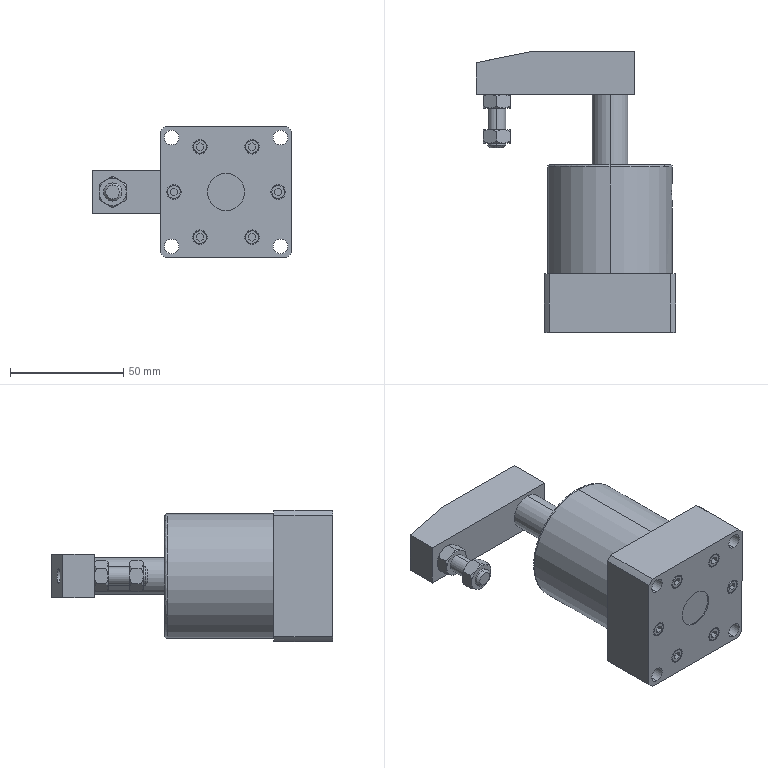Part | SolidWorks | 2 solids | 210 faces | box 88 x 124 x 58 mm | volume 194195 mm3 | plane 92 | cylinder 62 | cone 42 | spline 14 | commonest cylinder face diameters 6 x12 6.4 x12 6.5 x8 8 x4 8.566 x4 16 x4